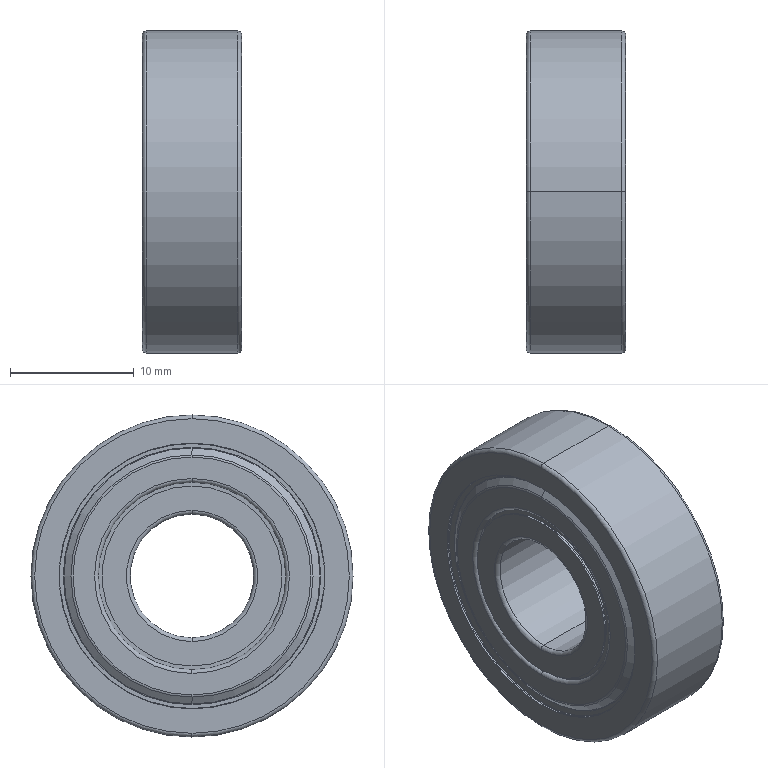Part | STEP file | ball bearing-B6000ZZ | 14 solids | 404 faces | box 8 x 26 x 26 mm | volume 2612 mm3 | sphere 144 | plane 106 | cylinder 88 | torus 38 | cone 28 | commonest cylinder face diameters 15.333 x8 22.267 x8 0.296 x7 0.516 x6 0.367 x5 0.441 x5